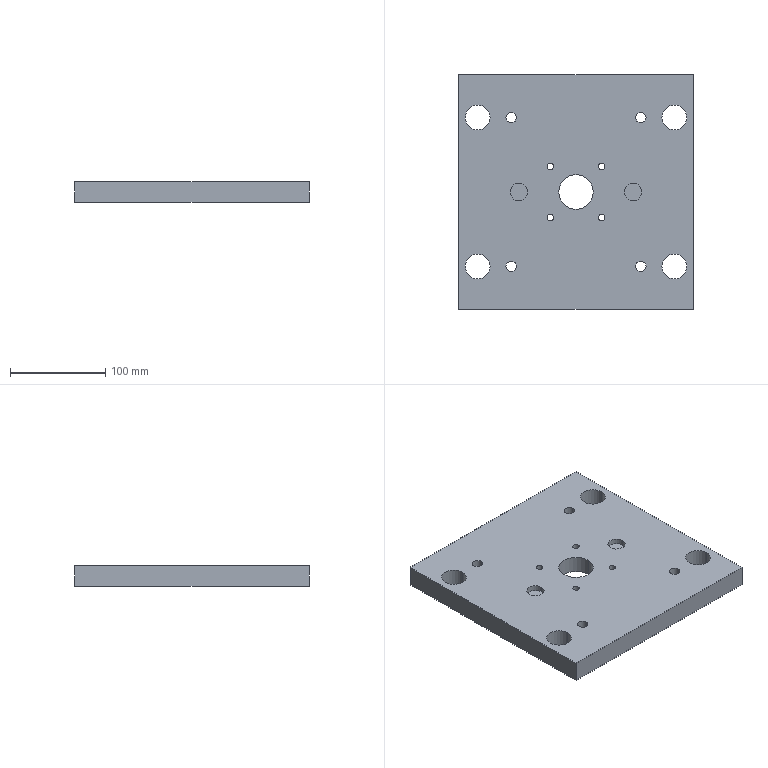Part | STEP file | 7 | 1 solid | 53 faces | box 246 x 246 x 22 mm | volume 1219815 mm3 | cylinder 40 | plane 13 | commonest cylinder face diameters 18 x12 6.8 x8 11 x8 26 x8 36 x2 90 x2